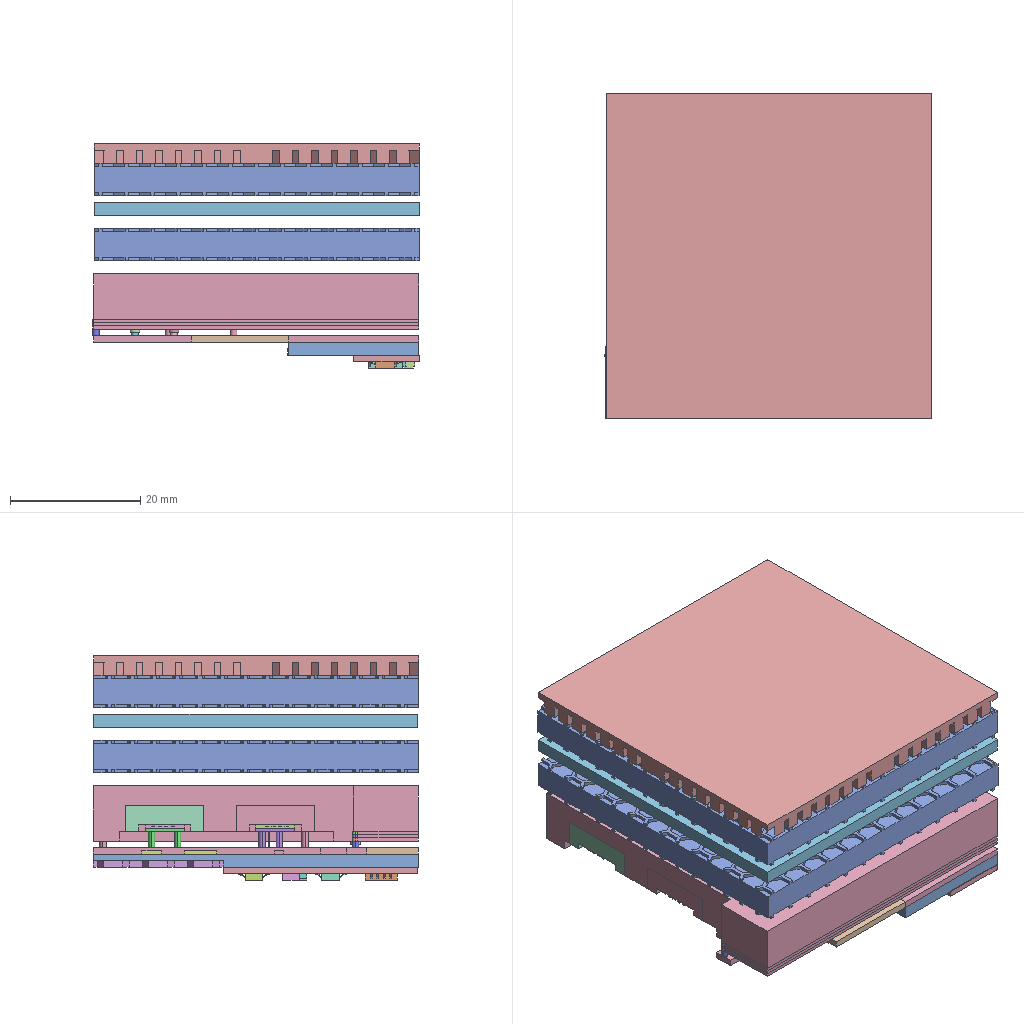Assembly | SolidWorks | 5 different items | 6 placed | box 50 x 50 x 34 mm
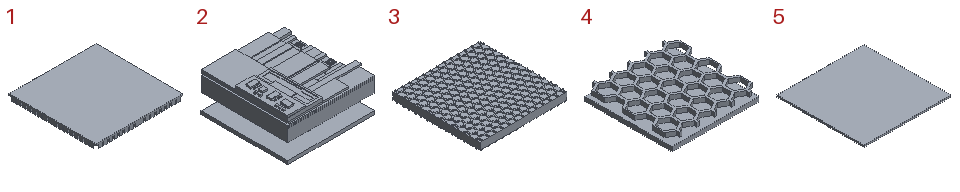Parts list (item | quantity | size | volume | features):
1 | x1 | 50 x 50 x 3 mm | 5676 mm3 | features ICE 2, Extrusion 1
2 | x1 | 50.25 x 50 x 25.5 mm | 28187 mm3 | features ICE 50, MoveCopyBody 5, LPattern 4, Split 3, Extrusion 1
3 | x2 | 50 x 50 x 5 mm | 10617 mm3 | features ICE 4, MirrorSolid 2, APattern 1, Extrusion 1
4 | x1 | 20 x 20 x 3 mm | 501.821 mm3 | features ICE 6, APattern 1, Extrusion 1
5 | x1 | 50 x 50 x 1 mm | 2500 mm3 | features Extrusion 1
Mates (type | each side: item.copy, entity, surface, feature):
DistanceDim | 3.1 face plane Boss-Extrude1 | 2.1 face plane Boss-Extrude6
Coincident | 1.1 face plane Boss-Extrude4 | 3.1 face plane Cut-Extrude1 | 2 times
Coincident | 1.1 face plane Boss-Extrude4 | 3.1 face plane Boss-Extrude1
Coincident | 2.1 face plane Boss-Extrude6 | 3.1 face plane Cut-Extrude1
Coincident | 2.1 face plane Boss-Extrude6 | 3.2 face plane Cut-Extrude1 | 2 times
DistanceDim | 3.2 face plane Boss-Extrude1 | 2.1 face plane Boss-Extrude7
Coincident | 2.1 face plane Cut-Extrude10 | 4.1 face plane Boss-Extrude1
Coincident | 1.1 face plane Boss-Extrude4 | 5.1 face plane Boss-Extrude1 | 2 times
DistanceDim | 5.1 face plane Boss-Extrude1 | 1.1 face plane Boss-Extrude4